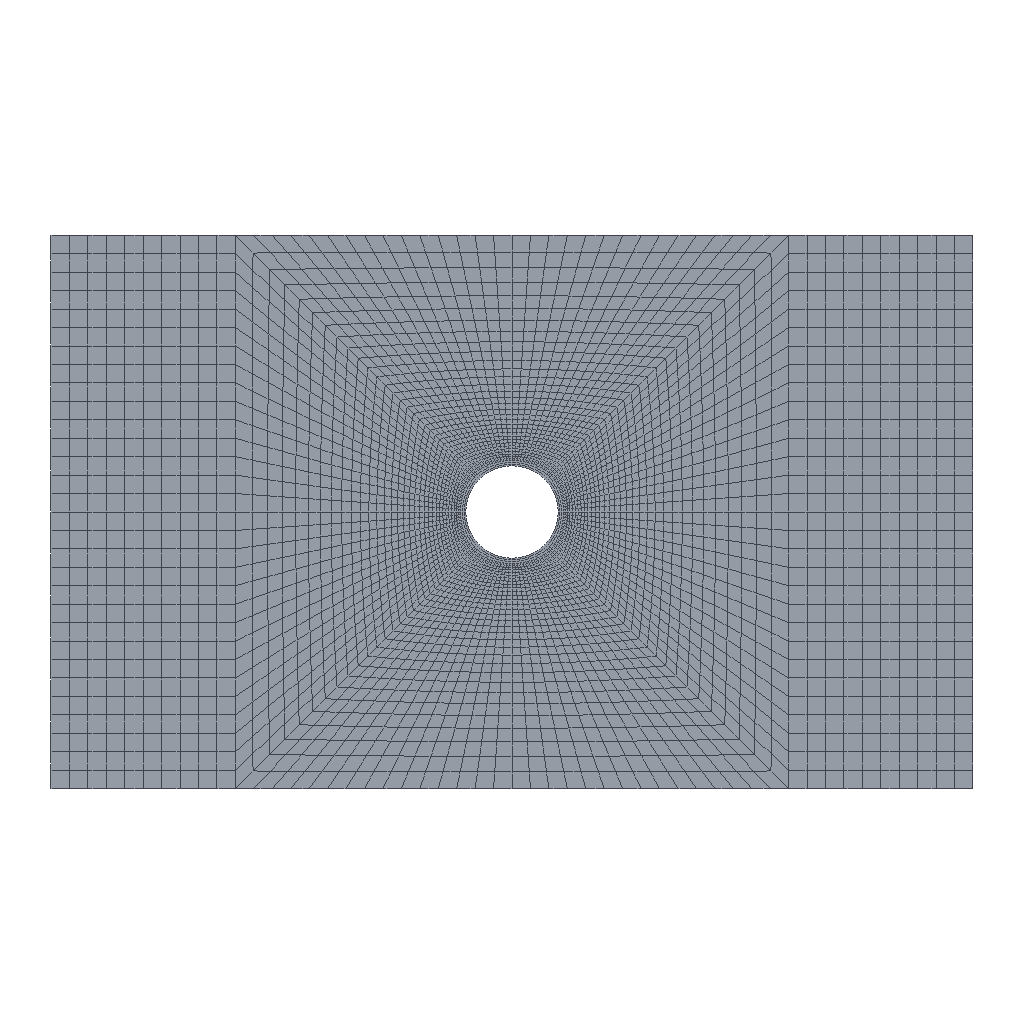Simulation study | abaqus
Set-up summary:
category,name,step,type,value,unit,region
solver,abaqus,,Abaqus/CAE 2024
units,mm-N-s-tonne (MPa),,inferred,E=114000 density=
analysis,Step-1,,static,time_period=1
mesh,nodes,,,4940
mesh,elements,,,4800
element_type,S4R,,,4800
material,Mat-T700,,E,114000
material,Mat-T700,,nu,0.3
material,Mat-T700,,behaviors,damage initiation; damage evolution; damage stabilization; elastic lamina
section,,,shell section,0.15,,CompositeLayup-1-1
bc,BC-Left,initial,encastre,[dofs=ENCASTRE],,_PickedSet40
bc,BC-Z,initial,fixed,[dofs=z],,_PickedSet38
bc,BC-X,Step-1,displacement,-1 [dofs=x],,Nd-1
bc,BC-X,Step-1,fixed,"[dofs=rx,ry,rz,y,z n=5]",,Nd-1
constraint,mpc,,,1
Abaqus input file, long lists of numbers shortened:
*Heading
** Job name: deck Model name: Model-1
** Generated by: Abaqus/CAE 2024
*Preprint, echo=NO, model=NO, history=NO, contact=NO
**
** PARTS
**
*Part, name=Lam-S
*Node
      1,          80.,          60.,           0.
      2,          80.,           0.,           0.
** (4938 more lines like these left out)
*Element, type=S4R
  1,   1,  13, 475,  88
  2,  13,  14, 476, 475
** (4798 more lines like these left out)
*Orientation, name=Ori-1
1., 0., 0., 0., 1., 0.
3, 0.
** Region: (CompositeLayup-1-1: Generated From Layup)
*Elset, elset=CompositeLayup-1-1, generate
    1,  4800,     1
** Section: CompositeLayup-1-1
*Shell Section, elset=CompositeLayup-1-1, composite, orientation=Ori-1, layup=CompositeLayup-1, symmetric
0.15, 3, Mat-T700, 0., Ply-1
0.15, 3, Mat-T700, 45., Ply-2
0.15, 3, Mat-T700, -45., Ply-3
0.15, 3, Mat-T700, 45., Ply-4
0.15, 3, Mat-T700, 90., Ply-5
0.15, 3, Mat-T700, -45., Ply-6
0.15, 3, Mat-T700, 0., Ply-7
0.15, 3, Mat-T700, 0., Ply-8
0.15, 3, Mat-T700, -45., Ply-9
0.15, 3, Mat-T700, 0., Ply-10
0.15, 3, Mat-T700, 0., Ply-11
0.15, 3, Mat-T700, 45., Ply-12
0.075, 3, Mat-T700, 90., Ply-13
*End Part
**
**
** ASSEMBLY
**
*Assembly, name=Assembly
**
*Instance, name=Lam-S-1, part=Lam-S
*End Instance
**
*Nset, nset=Nd-1, instance=Lam-S-1
 65,
*Nset, nset=_PickedSet38, internal, instance=Lam-S-1
   1,   2,   3,   4,   7,   8,   9,  10,  42,  43,  44,  45,  46,  47,  48,  49
  50,  80,  81,  82,  83,  84,  85,  86,  87,  88, 215, 216, 217, 218, 219, 220
** (5 more lines like these left out)
*Elset, elset=_PickedSet38, internal, instance=Lam-S-1
    1,   30,   31,   60,   61,   90,   91,  120,  121,  150,  151,  180,  181,  210,  211,  240
  241,  270,  271,  300, 1351, 1380, 1381, 1410, 1411, 1440, 1441, 1470, 1471, 1500, 1501, 1530
** (5 more lines like these left out)
*Nset, nset=_PickedSet39, internal, instance=Lam-S-1
  3,  4, 51, 52, 53, 54, 55, 56, 57, 58, 59, 60, 61, 62, 63, 64
 65, 66, 67, 68, 69, 70, 71, 72, 73, 74, 75, 76, 77, 78, 79
*Elset, elset=_PickedSet39, internal, instance=Lam-S-1, generate
 271,  300,    1
*Nset, nset=_PickedSet40, internal, instance=Lam-S-1
   9,  10, 224, 225, 226, 227, 228, 229, 230, 231, 232, 233, 234, 235, 236, 237
 238, 239, 240, 241, 242, 243, 244, 245, 246, 247, 248, 249, 250, 251, 252
*Elset, elset=_PickedSet40, internal, instance=Lam-S-1, generate
 1621,  1650,     1
*Surface, type=NODE, name=_PickedSet39_CNS_, internal
_PickedSet39, 1.
** Constraint: Constraint-1
*MPC
BEAM, _PickedSet39, Nd-1
*End Assembly
**
** MATERIALS
**
*Material, name=Mat-T700
*Damage Initiation, criterion=HASHIN
2688.,1458., 69.5, 236., 136., 95.6
*Damage Evolution, type=ENERGY
15.,15., 1., 1.
*Damage Stabilization
0.001,0.001,0.005,0.005
*Elastic, type=LAMINA
114000.,8610.,  0.3,4160.,4160.,3000.
**
** BOUNDARY CONDITIONS
**
** Name: BC-Left Type: Symmetry/Antisymmetry/Encastre
*Boundary
_PickedSet40, ENCASTRE
** Name: BC-Z Type: Displacement/Rotation
*Boundary
_PickedSet38, 3, 3
** ----------------------------------------------------------------
**
** STEP: Step-1
**
*Step, name=Step-1, nlgeom=NO, inc=1000
*Static
0.01, 1., 1e-15, 0.01
**
** BOUNDARY CONDITIONS
**
** Name: BC-X Type: Displacement/Rotation
*Boundary
Nd-1, 1, 1, -1.
Nd-1, 2, 2
Nd-1, 3, 3
Nd-1, 4, 4
Nd-1, 5, 5
Nd-1, 6, 6
**
** OUTPUT REQUESTS
**
*Restart, write, frequency=0
**
** FIELD OUTPUT: F-Output-2
**
*Output, field
*Node Output
U,
**
** FIELD OUTPUT: F-Output-1
**
*Output, field, time interval=0.02
*Element Output, elset=Lam-S-1.CompositeLayup-1-1, directions=YES
2, 5, 8, 11, 14, 17, 20, 23, 26, 29, 32, 35, 38, 41, 44, 47
DAMAGEFC, DAMAGEFT, DAMAGEMC, DAMAGEMT, E, HSNFCCRT, HSNFTCRT, HSNMCCRT, HSNMTCRT, S
*Element Output, elset=Lam-S-1.CompositeLayup-1-1, directions=YES
50, 53, 56, 59, 62, 65, 68, 71, 74, 77
DAMAGEFC, DAMAGEFT, DAMAGEMC, DAMAGEMT, E, HSNFCCRT, HSNFTCRT, HSNMCCRT, HSNMTCRT, S
**
** HISTORY OUTPUT: H-Output-1
**
*Output, history, time interval=0.01
*Node Output, nset=Nd-1
RF1, U1
*End Step
Results summary:
result,odb.job_status,,,JOB_STATUS_COMPLETED_SUCCESSFULLY,"consistent, unstated (Abaqus has no unit system)"
result,steps[0].procedure,Step-1,,*STATIC,"consistent, unstated (Abaqus has no unit system)"
result,steps[0].time_period,Step-1,,1,"consistent, unstated (Abaqus has no unit system)"
result,steps[0].n_frames,Step-1,,210,"consistent, unstated (Abaqus has no unit system)"
result,steps[0].last_frame.id,Step-1,,209,"consistent, unstated (Abaqus has no unit system)"
result,steps[0].last_frame.value,Step-1,,1,"consistent, unstated (Abaqus has no unit system)"
result,steps[0].last_frame.description,Step-1,,Increment    209: Step Time =    1.000,"consistent, unstated (Abaqus has no unit system)"
result,steps[0].completed,Step-1,,True,"consistent, unstated (Abaqus has no unit system)"
result,steps[0].max_U_magnitude,Step-1,,1,"consistent, unstated (Abaqus has no unit system)"
result,steps[0].max_S_mises,Step-1,,1401.45,"consistent, unstated (Abaqus has no unit system)"
result,steps[0].diagnostic.n_increments,Step-1,,209,"consistent, unstated (Abaqus has no unit system)"